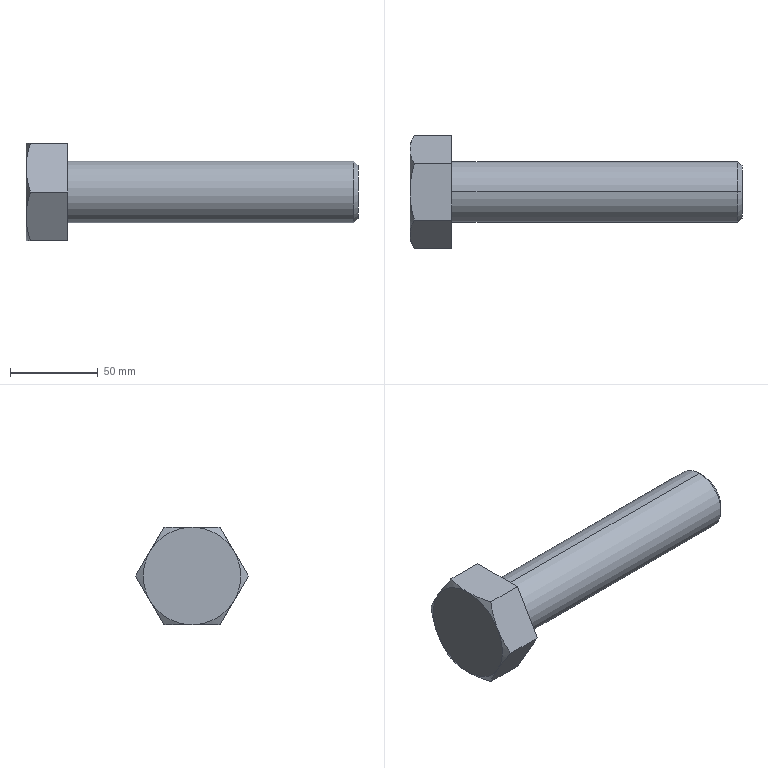Part | SolidWorks | features RevCut 2, Extrusion 1, Fillet 1, LPattern 1, Revolution 1 | 1 solid | 19 faces | box 188.976 x 64.173 x 55.575 mm | volume 221511 mm3 | plane 9 | cone 8 | cylinder 2 | commonest cylinder face diameters 34.925 x2
STEP:
#1=CARTESIAN_POINT('',(7.44,0.,0.5883));
#2=VERTEX_POINT('',#1);
#3=CARTESIAN_POINT('',(7.44,0.,-0.5883));
#4=VERTEX_POINT('',#3);
#5=CARTESIAN_POINT('',(7.44,0.,0.));
#6=DIRECTION('',(-1.,0.,0.));
#7=DIRECTION('',(0.,0.,1.));
#8=AXIS2_PLACEMENT_3D('',#5,#6,#7);
#9=CIRCLE('',#8,0.5883);
#10=EDGE_CURVE('',#2,#4,#9,.T.);
#11=ORIENTED_EDGE('',*,*,#10,.T.);
#12=CARTESIAN_POINT('',(7.341,0.,-0.6875));
#13=VERTEX_POINT('',#12);
#14=CARTESIAN_POINT('',(7.44,0.,-0.5883));
#15=DIRECTION('',(-0.7071,0.,-0.7071));
#16=VECTOR('',#15,39.37);
#17=LINE('',#14,#16);
#18=EDGE_CURVE('',#4,#13,#17,.T.);
#19=ORIENTED_EDGE('',*,*,#18,.T.);
#20=CARTESIAN_POINT('',(7.341,0.,0.6875));
#21=VERTEX_POINT('',#20);
#22=CARTESIAN_POINT('',(7.341,0.,0.));
#23=DIRECTION('',(-1.,0.,0.));
#24=DIRECTION('',(0.,0.,1.));
#25=AXIS2_PLACEMENT_3D('',#22,#23,#24);
#26=CIRCLE('',#25,0.6875);
#27=EDGE_CURVE('',#21,#13,#26,.T.);
#28=ORIENTED_EDGE('',*,*,#27,.F.);
#29=CARTESIAN_POINT('',(7.44,0.,0.5883));
#30=DIRECTION('',(-0.7071,0.,0.7071));
#31=VECTOR('',#30,39.37);
#32=LINE('',#29,#31);
#33=EDGE_CURVE('',#2,#21,#32,.T.);
#34=ORIENTED_EDGE('',*,*,#33,.F.);
#35=EDGE_LOOP('',(#11,#19,#28,#34));
#36=FACE_OUTER_BOUND('',#35,.T.);
#37=CARTESIAN_POINT('',(7.44,0.,0.));
#38=DIRECTION('',(-1.,0.,0.));
#39=DIRECTION('',(0.,0.,1.));
#40=AXIS2_PLACEMENT_3D('',#37,#38,#39);
#41=CONICAL_SURFACE('',#40,0.5883,0.7854);
#42=ADVANCED_FACE('',(#36),#41,.T.);
#43=ORIENTED_EDGE('',*,*,#27,.T.);
#44=CARTESIAN_POINT('',(0.94,0.,-0.6875));
#45=VERTEX_POINT('',#44);
#46=CARTESIAN_POINT('',(0.,0.,-0.6875));
#47=DIRECTION('',(-1.,0.,0.));
#48=VECTOR('',#47,39.37);
#49=LINE('',#46,#48);
#50=EDGE_CURVE('',#13,#45,#49,.T.);
#51=ORIENTED_EDGE('',*,*,#50,.T.);
#52=CARTESIAN_POINT('',(0.94,0.,0.6875));
#53=VERTEX_POINT('',#52);
#54=CARTESIAN_POINT('',(0.94,0.,0.));
#55=DIRECTION('',(-1.,0.,0.));
#56=DIRECTION('',(0.,0.,-1.));
#57=AXIS2_PLACEMENT_3D('',#54,#55,#56);
#58=CIRCLE('',#57,0.6875);
#59=EDGE_CURVE('',#53,#45,#58,.T.);
#60=ORIENTED_EDGE('',*,*,#59,.F.);
#61=CARTESIAN_POINT('',(0.,0.,0.6875));
#62=DIRECTION('',(-1.,0.,0.));
#63=VECTOR('',#62,39.37);
#64=LINE('',#61,#63);
#65=EDGE_CURVE('',#21,#53,#64,.T.);
#66=ORIENTED_EDGE('',*,*,#65,.F.);
#67=EDGE_LOOP('',(#43,#51,#60,#66));
#68=FACE_OUTER_BOUND('',#67,.T.);
#69=CARTESIAN_POINT('',(0.,0.,0.));
#70=DIRECTION('',(-1.,0.,0.));
#71=DIRECTION('',(0.,0.,1.));
#72=AXIS2_PLACEMENT_3D('',#69,#70,#71);
#73=CYLINDRICAL_SURFACE('',#72,0.6875);
#74=ADVANCED_FACE('',(#68),#73,.T.);
#75=CARTESIAN_POINT('',(0.09771,1.263,0.));
#76=VERTEX_POINT('',#75);
#77=CARTESIAN_POINT('',(0.,0.9474,-0.547));
#78=VERTEX_POINT('',#77);
#79=CARTESIAN_POINT('',(0.09771,1.263,0.));
#80=CARTESIAN_POINT('',(0.06788,1.212,-0.08948));
#81=CARTESIAN_POINT('',(0.04331,1.16,-0.1796));
#82=CARTESIAN_POINT('',(0.009312,1.054,-0.3618));
#83=CARTESIAN_POINT('',(0.,1.001,-0.4538));
#84=CARTESIAN_POINT('',(0.,0.9474,-0.547));
#85=B_SPLINE_CURVE_WITH_KNOTS('',3,(#79,#80,#81,#82,#83,#84),.UNSPECIFIED.,.F.,.F.,(4,2,4),(0.000000238,0.008117,0.01623),.UNSPECIFIED.);
#86=EDGE_CURVE('',#76,#78,#85,.T.);
#87=ORIENTED_EDGE('',*,*,#86,.F.);
#88=CARTESIAN_POINT('',(0.94,1.263,0.));
#89=VERTEX_POINT('',#88);
#90=CARTESIAN_POINT('',(0.94,1.263,0.));
#91=DIRECTION('',(-1.,0.,0.));
#92=VECTOR('',#91,39.37);
#93=LINE('',#90,#92);
#94=EDGE_CURVE('',#89,#76,#93,.T.);
#95=ORIENTED_EDGE('',*,*,#94,.F.);
#96=CARTESIAN_POINT('',(0.94,0.6316,-1.094));
#97=VERTEX_POINT('',#96);
#98=CARTESIAN_POINT('',(0.94,0.6316,-1.094));
#99=DIRECTION('',(0.,0.5,0.866));
#100=VECTOR('',#99,39.37);
#101=LINE('',#98,#100);
#102=EDGE_CURVE('',#97,#89,#101,.T.);
#103=ORIENTED_EDGE('',*,*,#102,.F.);
#104=CARTESIAN_POINT('',(0.09771,0.6316,-1.094));
#105=VERTEX_POINT('',#104);
#106=CARTESIAN_POINT('',(0.94,0.6316,-1.094));
#107=DIRECTION('',(-1.,0.,0.));
#108=VECTOR('',#107,39.37);
#109=LINE('',#106,#108);
#110=EDGE_CURVE('',#97,#105,#109,.T.);
#111=ORIENTED_EDGE('',*,*,#110,.T.);
#112=CARTESIAN_POINT('',(0.,0.9474,-0.547));
#113=CARTESIAN_POINT('',(0.,0.934,-0.5702));
#114=CARTESIAN_POINT('',(0.0005731,0.9206,-0.5935));
#115=CARTESIAN_POINT('',(0.002846,0.8938,-0.64));
#116=CARTESIAN_POINT('',(0.004544,0.8804,-0.6631));
#117=CARTESIAN_POINT('',(0.01125,0.8405,-0.7323));
#118=CARTESIAN_POINT('',(0.01787,0.814,-0.7781));
#119=CARTESIAN_POINT('',(0.0434,0.7351,-0.9147));
#120=CARTESIAN_POINT('',(0.06796,0.6832,-1.005));
#121=CARTESIAN_POINT('',(0.09771,0.6316,-1.094));
#122=B_SPLINE_CURVE_WITH_KNOTS('',3,(#112,#113,#114,#115,#116,#117,#118,#119,#120,#121),.UNSPECIFIED.,.F.,.F.,(4,2,2,2,4),(0.01623,0.01825,0.02028,0.02432,0.03241),.UNSPECIFIED.);
#123=EDGE_CURVE('',#78,#105,#122,.T.);
#124=ORIENTED_EDGE('',*,*,#123,.F.);
#125=EDGE_LOOP('',(#87,#95,#103,#111,#124));
#126=FACE_OUTER_BOUND('',#125,.T.);
#127=CARTESIAN_POINT('',(0.94,0.6316,-1.094));
#128=DIRECTION('',(0.,-0.866,0.5));
#129=DIRECTION('',(0.,-0.5,-0.866));
#130=AXIS2_PLACEMENT_3D('',#127,#128,#129);
#131=PLANE('',#130);
#132=ADVANCED_FACE('',(#126),#131,.F.);
#133=CARTESIAN_POINT('',(0.09771,0.6316,1.094));
#134=VERTEX_POINT('',#133);
#135=CARTESIAN_POINT('',(0.,0.9474,0.547));
#136=VERTEX_POINT('',#135);
#137=CARTESIAN_POINT('',(0.09771,0.6316,1.094));
#138=CARTESIAN_POINT('',(0.06788,0.6833,1.005));
#139=CARTESIAN_POINT('',(0.04331,0.7353,0.9144));
#140=CARTESIAN_POINT('',(0.009312,0.8405,0.7322));
#141=CARTESIAN_POINT('',(0.,0.8936,0.6402));
#142=CARTESIAN_POINT('',(0.,0.9474,0.547));
#143=B_SPLINE_CURVE_WITH_KNOTS('',3,(#137,#138,#139,#140,#141,#142),.UNSPECIFIED.,.F.,.F.,(4,2,4),(0.000000238,0.008117,0.01623),.UNSPECIFIED.);
#144=EDGE_CURVE('',#134,#136,#143,.T.);
#145=ORIENTED_EDGE('',*,*,#144,.F.);
#146=CARTESIAN_POINT('',(0.94,0.6316,1.094));
#147=VERTEX_POINT('',#146);
#148=CARTESIAN_POINT('',(0.94,0.6316,1.094));
#149=DIRECTION('',(-1.,0.,0.));
#150=VECTOR('',#149,39.37);
#151=LINE('',#148,#150);
#152=EDGE_CURVE('',#147,#134,#151,.T.);
#153=ORIENTED_EDGE('',*,*,#152,.F.);
#154=CARTESIAN_POINT('',(0.94,1.263,0.));
#155=DIRECTION('',(0.,-0.5,0.866));
#156=VECTOR('',#155,39.37);
#157=LINE('',#154,#156);
#158=EDGE_CURVE('',#89,#147,#157,.T.);
#159=ORIENTED_EDGE('',*,*,#158,.F.);
#160=ORIENTED_EDGE('',*,*,#94,.T.);
#161=CARTESIAN_POINT('',(0.,0.9474,0.547));
#162=CARTESIAN_POINT('',(0.,0.9608,0.5238));
#163=CARTESIAN_POINT('',(0.0005731,0.9743,0.5005));
#164=CARTESIAN_POINT('',(0.002846,1.001,0.454));
#165=CARTESIAN_POINT('',(0.004544,1.014,0.4309));
#166=CARTESIAN_POINT('',(0.01125,1.054,0.3617));
#167=CARTESIAN_POINT('',(0.01787,1.081,0.3159));
#168=CARTESIAN_POINT('',(0.0434,1.16,0.1793));
#169=CARTESIAN_POINT('',(0.06796,1.212,0.08926));
#170=CARTESIAN_POINT('',(0.09771,1.263,0.));
#171=B_SPLINE_CURVE_WITH_KNOTS('',3,(#161,#162,#163,#164,#165,#166,#167,#168,#169,#170),.UNSPECIFIED.,.F.,.F.,(4,2,2,2,4),(0.01623,0.01825,0.02028,0.02432,0.03241),.UNSPECIFIED.);
#172=EDGE_CURVE('',#136,#76,#171,.T.);
#173=ORIENTED_EDGE('',*,*,#172,.F.);
#174=EDGE_LOOP('',(#145,#153,#159,#160,#173));
#175=FACE_OUTER_BOUND('',#174,.T.);
#176=CARTESIAN_POINT('',(0.94,1.263,0.));
#177=DIRECTION('',(0.,-0.866,-0.5));
#178=DIRECTION('',(0.,0.5,-0.866));
#179=AXIS2_PLACEMENT_3D('',#176,#177,#178);
#180=PLANE('',#179);
#181=ADVANCED_FACE('',(#175),#180,.F.);
#182=CARTESIAN_POINT('',(0.09771,-0.6316,1.094));
#183=VERTEX_POINT('',#182);
#184=CARTESIAN_POINT('',(0.,0.,1.094));
#185=VERTEX_POINT('',#184);
#186=CARTESIAN_POINT('',(0.09771,-0.6316,1.094));
#187=CARTESIAN_POINT('',(0.08288,-0.5802,1.094));
#188=CARTESIAN_POINT('',(0.06924,-0.5283,1.094));
#189=CARTESIAN_POINT('',(0.0451,-0.4235,1.094));
#190=CARTESIAN_POINT('',(0.03468,-0.3709,1.094));
#191=CARTESIAN_POINT('',(0.009184,-0.2128,1.094));
#192=CARTESIAN_POINT('',(0.,-0.1068,1.094));
#193=CARTESIAN_POINT('',(0.,0.,1.094));
#194=B_SPLINE_CURVE_WITH_KNOTS('',3,(#186,#187,#188,#189,#190,#191,#192,#193),.UNSPECIFIED.,.F.,.F.,(4,2,2,4),(0.02919,0.03325,0.03731,0.04543),.UNSPECIFIED.);
#195=EDGE_CURVE('',#183,#185,#194,.T.);
#196=ORIENTED_EDGE('',*,*,#195,.F.);
#197=CARTESIAN_POINT('',(0.94,-0.6316,1.094));
#198=VERTEX_POINT('',#197);
#199=CARTESIAN_POINT('',(0.94,-0.6316,1.094));
#200=DIRECTION('',(-1.,0.,0.));
#201=VECTOR('',#200,39.37);
#202=LINE('',#199,#201);
#203=EDGE_CURVE('',#198,#183,#202,.T.);
#204=ORIENTED_EDGE('',*,*,#203,.F.);
#205=CARTESIAN_POINT('',(0.94,0.6316,1.094));
#206=DIRECTION('',(0.,-1.,0.));
#207=VECTOR('',#206,39.37);
#208=LINE('',#205,#207);
#209=EDGE_CURVE('',#147,#198,#208,.T.);
#210=ORIENTED_EDGE('',*,*,#209,.F.);
#211=ORIENTED_EDGE('',*,*,#152,.T.);
#212=CARTESIAN_POINT('',(0.,0.,1.094));
#213=CARTESIAN_POINT('',(0.,0.05344,1.094));
#214=CARTESIAN_POINT('',(0.002274,0.1071,1.094));
#215=CARTESIAN_POINT('',(0.01131,0.2147,1.094));
#216=CARTESIAN_POINT('',(0.018,0.2679,1.094));
#217=CARTESIAN_POINT('',(0.04368,0.426,1.094));
#218=CARTESIAN_POINT('',(0.06823,0.5295,1.094));
#219=CARTESIAN_POINT('',(0.09771,0.6316,1.094));
#220=B_SPLINE_CURVE_WITH_KNOTS('',3,(#212,#213,#214,#215,#216,#217,#218,#219),.UNSPECIFIED.,.F.,.F.,(4,2,2,4),(0.04543,0.04949,0.05355,0.06167),.UNSPECIFIED.);
#221=EDGE_CURVE('',#185,#134,#220,.T.);
#222=ORIENTED_EDGE('',*,*,#221,.F.);
#223=EDGE_LOOP('',(#196,#204,#210,#211,#222));
#224=FACE_OUTER_BOUND('',#223,.T.);
#225=CARTESIAN_POINT('',(0.94,0.6316,1.094));
#226=DIRECTION('',(0.,0.,-1.));
#227=DIRECTION('',(0.,1.,0.));
#228=AXIS2_PLACEMENT_3D('',#225,#226,#227);
#229=PLANE('',#228);
#230=ADVANCED_FACE('',(#224),#229,.F.);
#231=CARTESIAN_POINT('',(0.09771,-1.263,0.));
#232=VERTEX_POINT('',#231);
#233=CARTESIAN_POINT('',(0.,-0.9474,0.547));
#234=VERTEX_POINT('',#233);
#235=CARTESIAN_POINT('',(0.09771,-1.263,0.));
#236=CARTESIAN_POINT('',(0.06788,-1.212,0.08948));
#237=CARTESIAN_POINT('',(0.04331,-1.16,0.1796));
#238=CARTESIAN_POINT('',(0.009312,-1.054,0.3618));
#239=CARTESIAN_POINT('',(0.,-1.001,0.4538));
#240=CARTESIAN_POINT('',(0.,-0.9474,0.547));
#241=B_SPLINE_CURVE_WITH_KNOTS('',3,(#235,#236,#237,#238,#239,#240),.UNSPECIFIED.,.F.,.F.,(4,2,4),(0.000000238,0.008117,0.01623),.UNSPECIFIED.);
#242=EDGE_CURVE('',#232,#234,#241,.T.);
#243=ORIENTED_EDGE('',*,*,#242,.F.);
#244=CARTESIAN_POINT('',(0.94,-1.263,0.));
#245=VERTEX_POINT('',#244);
#246=CARTESIAN_POINT('',(0.94,-1.263,0.));
#247=DIRECTION('',(-1.,0.,0.));
#248=VECTOR('',#247,39.37);
#249=LINE('',#246,#248);
#250=EDGE_CURVE('',#245,#232,#249,.T.);
#251=ORIENTED_EDGE('',*,*,#250,.F.);
#252=CARTESIAN_POINT('',(0.94,-1.263,0.));
#253=DIRECTION('',(0.,-0.5,-0.866));
#254=VECTOR('',#253,39.37);
#255=LINE('',#252,#254);
#256=EDGE_CURVE('',#198,#245,#255,.T.);
#257=ORIENTED_EDGE('',*,*,#256,.F.);
#258=ORIENTED_EDGE('',*,*,#203,.T.);
#259=CARTESIAN_POINT('',(0.,-0.9474,0.547));
#260=CARTESIAN_POINT('',(0.,-0.934,0.5702));
#261=CARTESIAN_POINT('',(0.0005731,-0.9206,0.5935));
#262=CARTESIAN_POINT('',(0.002846,-0.8938,0.64));
#263=CARTESIAN_POINT('',(0.004544,-0.8804,0.6631));
#264=CARTESIAN_POINT('',(0.01125,-0.8405,0.7323));
#265=CARTESIAN_POINT('',(0.01787,-0.814,0.7781));
#266=CARTESIAN_POINT('',(0.0434,-0.7351,0.9147));
#267=CARTESIAN_POINT('',(0.06796,-0.6832,1.005));
#268=CARTESIAN_POINT('',(0.09771,-0.6316,1.094));
#269=B_SPLINE_CURVE_WITH_KNOTS('',3,(#259,#260,#261,#262,#263,#264,#265,#266,#267,#268),.UNSPECIFIED.,.F.,.F.,(4,2,2,2,4),(0.01623,0.01825,0.02028,0.02432,0.03241),.UNSPECIFIED.);
#270=EDGE_CURVE('',#234,#183,#269,.T.);
#271=ORIENTED_EDGE('',*,*,#270,.F.);
#272=EDGE_LOOP('',(#243,#251,#257,#258,#271));
#273=FACE_OUTER_BOUND('',#272,.T.);
#274=CARTESIAN_POINT('',(0.94,-1.263,0.));
#275=DIRECTION('',(0.,0.866,-0.5));
#276=DIRECTION('',(0.,0.5,0.866));
#277=AXIS2_PLACEMENT_3D('',#274,#275,#276);
#278=PLANE('',#277);
#279=ADVANCED_FACE('',(#273),#278,.F.);
#280=CARTESIAN_POINT('',(0.09771,-0.6316,-1.094));
#281=VERTEX_POINT('',#280);
#282=CARTESIAN_POINT('',(0.,-0.9474,-0.547));
#283=VERTEX_POINT('',#282);
#284=CARTESIAN_POINT('',(0.09771,-0.6316,-1.094));
#285=CARTESIAN_POINT('',(0.06788,-0.6833,-1.005));
#286=CARTESIAN_POINT('',(0.04331,-0.7353,-0.9144));
#287=CARTESIAN_POINT('',(0.009312,-0.8405,-0.7322));
#288=CARTESIAN_POINT('',(0.,-0.8936,-0.6402));
#289=CARTESIAN_POINT('',(0.,-0.9474,-0.547));
#290=B_SPLINE_CURVE_WITH_KNOTS('',3,(#284,#285,#286,#287,#288,#289),.UNSPECIFIED.,.F.,.F.,(4,2,4),(0.000000238,0.008117,0.01623),.UNSPECIFIED.);
#291=EDGE_CURVE('',#281,#283,#290,.T.);
#292=ORIENTED_EDGE('',*,*,#291,.F.);
#293=CARTESIAN_POINT('',(0.94,-0.6316,-1.094));
#294=VERTEX_POINT('',#293);
#295=CARTESIAN_POINT('',(0.94,-0.6316,-1.094));
#296=DIRECTION('',(-1.,0.,0.));
#297=VECTOR('',#296,39.37);
#298=LINE('',#295,#297);
#299=EDGE_CURVE('',#294,#281,#298,.T.);
#300=ORIENTED_EDGE('',*,*,#299,.F.);
#301=CARTESIAN_POINT('',(0.94,-0.6316,-1.094));
#302=DIRECTION('',(0.,0.5,-0.866));
#303=VECTOR('',#302,39.37);
#304=LINE('',#301,#303);
#305=EDGE_CURVE('',#245,#294,#304,.T.);
#306=ORIENTED_EDGE('',*,*,#305,.F.);
#307=ORIENTED_EDGE('',*,*,#250,.T.);
#308=CARTESIAN_POINT('',(0.,-0.9474,-0.547));
#309=CARTESIAN_POINT('',(0.,-0.9608,-0.5238));
#310=CARTESIAN_POINT('',(0.0005731,-0.9743,-0.5005));
#311=CARTESIAN_POINT('',(0.002846,-1.001,-0.454));
#312=CARTESIAN_POINT('',(0.004544,-1.014,-0.4309));
#313=CARTESIAN_POINT('',(0.01125,-1.054,-0.3617));
#314=CARTESIAN_POINT('',(0.01787,-1.081,-0.3159));
#315=CARTESIAN_POINT('',(0.0434,-1.16,-0.1793));
#316=CARTESIAN_POINT('',(0.06796,-1.212,-0.08926));
#317=CARTESIAN_POINT('',(0.09771,-1.263,0.));
#318=B_SPLINE_CURVE_WITH_KNOTS('',3,(#308,#309,#310,#311,#312,#313,#314,#315,#316,#317),.UNSPECIFIED.,.F.,.F.,(4,2,2,2,4),(0.01623,0.01825,0.02028,0.02432,0.03241),.UNSPECIFIED.);
#319=EDGE_CURVE('',#283,#232,#318,.T.);
#320=ORIENTED_EDGE('',*,*,#319,.F.);
#321=EDGE_LOOP('',(#292,#300,#306,#307,#320));
#322=FACE_OUTER_BOUND('',#321,.T.);
#323=CARTESIAN_POINT('',(0.94,-0.6316,-1.094));
#324=DIRECTION('',(0.,0.866,0.5));
#325=DIRECTION('',(0.,-0.5,0.866));
#326=AXIS2_PLACEMENT_3D('',#323,#324,#325);
#327=PLANE('',#326);
#328=ADVANCED_FACE('',(#322),#327,.F.);
#329=CARTESIAN_POINT('',(0.,0.,-1.094));
#330=VERTEX_POINT('',#329);
#331=CARTESIAN_POINT('',(0.09771,0.6316,-1.094));
#332=CARTESIAN_POINT('',(0.06823,0.5295,-1.094));
#333=CARTESIAN_POINT('',(0.04368,0.426,-1.094));
#334=CARTESIAN_POINT('',(0.018,0.2679,-1.094));
#335=CARTESIAN_POINT('',(0.01131,0.2147,-1.094));
#336=CARTESIAN_POINT('',(0.002274,0.1071,-1.094));
#337=CARTESIAN_POINT('',(0.,0.05344,-1.094));
#338=CARTESIAN_POINT('',(0.,0.,-1.094));
#339=B_SPLINE_CURVE_WITH_KNOTS('',3,(#331,#332,#333,#334,#335,#336,#337,#338),.UNSPECIFIED.,.F.,.F.,(4,2,2,4),(0.07205,0.08018,0.08424,0.08831),.UNSPECIFIED.);
#340=EDGE_CURVE('',#105,#330,#339,.T.);
#341=ORIENTED_EDGE('',*,*,#340,.F.);
#342=ORIENTED_EDGE('',*,*,#110,.F.);
#343=CARTESIAN_POINT('',(0.94,0.6316,-1.094));
#344=DIRECTION('',(0.,1.,0.));
#345=VECTOR('',#344,39.37);
#346=LINE('',#343,#345);
#347=EDGE_CURVE('',#294,#97,#346,.T.);
#348=ORIENTED_EDGE('',*,*,#347,.F.);
#349=ORIENTED_EDGE('',*,*,#299,.T.);
#350=CARTESIAN_POINT('',(0.,0.,-1.094));
#351=CARTESIAN_POINT('',(0.,-0.1068,-1.094));
#352=CARTESIAN_POINT('',(0.009184,-0.2128,-1.094));
#353=CARTESIAN_POINT('',(0.03468,-0.3709,-1.094));
#354=CARTESIAN_POINT('',(0.0451,-0.4235,-1.094));
#355=CARTESIAN_POINT('',(0.06924,-0.5283,-1.094));
#356=CARTESIAN_POINT('',(0.08288,-0.5802,-1.094));
#357=CARTESIAN_POINT('',(0.09771,-0.6316,-1.094));
#358=B_SPLINE_CURVE_WITH_KNOTS('',3,(#350,#351,#352,#353,#354,#355,#356,#357),.UNSPECIFIED.,.F.,.F.,(4,2,2,4),(0.08831,0.09643,0.1005,0.1046),.UNSPECIFIED.);
#359=EDGE_CURVE('',#330,#281,#358,.T.);
#360=ORIENTED_EDGE('',*,*,#359,.F.);
#361=EDGE_LOOP('',(#341,#342,#348,#349,#360));
#362=FACE_OUTER_BOUND('',#361,.T.);
#363=CARTESIAN_POINT('',(0.94,0.6316,-1.094));
#364=DIRECTION('',(0.,0.,1.));
#365=DIRECTION('',(0.,-1.,0.));
#366=AXIS2_PLACEMENT_3D('',#363,#364,#365);
#367=PLANE('',#366);
#368=ADVANCED_FACE('',(#362),#367,.F.);
#369=ORIENTED_EDGE('',*,*,#59,.T.);
#370=CARTESIAN_POINT('',(0.94,0.,0.));
#371=DIRECTION('',(-1.,0.,0.));
#372=DIRECTION('',(0.,0.,-1.));
#373=AXIS2_PLACEMENT_3D('',#370,#371,#372);
#374=CIRCLE('',#373,0.6875);
#375=EDGE_CURVE('',#45,#53,#374,.T.);
#376=ORIENTED_EDGE('',*,*,#375,.T.);
#377=EDGE_LOOP('',(#369,#376));
#378=FACE_BOUND('',#377,.T.);
#379=ORIENTED_EDGE('',*,*,#102,.T.);
#380=ORIENTED_EDGE('',*,*,#158,.T.);
#381=ORIENTED_EDGE('',*,*,#209,.T.);
#382=ORIENTED_EDGE('',*,*,#256,.T.);
#383=ORIENTED_EDGE('',*,*,#305,.T.);
#384=ORIENTED_EDGE('',*,*,#347,.T.);
#385=EDGE_LOOP('',(#379,#380,#381,#382,#383,#384));
#386=FACE_OUTER_BOUND('',#385,.T.);
#387=CARTESIAN_POINT('',(0.94,1.263,0.));
#388=DIRECTION('',(1.,0.,0.));
#389=DIRECTION('',(0.,0.,-1.));
#390=AXIS2_PLACEMENT_3D('',#387,#388,#389);
#391=PLANE('',#390);
#392=ADVANCED_FACE('',(#378,#386),#391,.T.);
#393=ORIENTED_EDGE('',*,*,#50,.F.);
#394=CARTESIAN_POINT('',(7.341,0.,0.));
#395=DIRECTION('',(-1.,0.,0.));
#396=DIRECTION('',(0.,0.,1.));
#397=AXIS2_PLACEMENT_3D('',#394,#395,#396);
#398=CIRCLE('',#397,0.6875);
#399=EDGE_CURVE('',#13,#21,#398,.T.);
#400=ORIENTED_EDGE('',*,*,#399,.T.);
#401=ORIENTED_EDGE('',*,*,#65,.T.);
#402=ORIENTED_EDGE('',*,*,#375,.F.);
#403=EDGE_LOOP('',(#393,#400,#401,#402));
#404=FACE_OUTER_BOUND('',#403,.T.);
#405=CARTESIAN_POINT('',(0.,0.,0.));
#406=DIRECTION('',(-1.,0.,0.));
#407=DIRECTION('',(0.,0.,1.));
#408=AXIS2_PLACEMENT_3D('',#405,#406,#407);
#409=CYLINDRICAL_SURFACE('',#408,0.6875);
#410=ADVANCED_FACE('',(#404),#409,.T.);
#411=ORIENTED_EDGE('',*,*,#18,.F.);
#412=CARTESIAN_POINT('',(7.44,0.,0.));
#413=DIRECTION('',(-1.,0.,0.));
#414=DIRECTION('',(0.,0.,1.));
#415=AXIS2_PLACEMENT_3D('',#412,#413,#414);
#416=CIRCLE('',#415,0.5883);
#417=EDGE_CURVE('',#4,#2,#416,.T.);
#418=ORIENTED_EDGE('',*,*,#417,.T.);
#419=ORIENTED_EDGE('',*,*,#33,.T.);
#420=ORIENTED_EDGE('',*,*,#399,.F.);
#421=EDGE_LOOP('',(#411,#418,#419,#420));
#422=FACE_OUTER_BOUND('',#421,.T.);
#423=CARTESIAN_POINT('',(7.44,0.,0.));
#424=DIRECTION('',(-1.,0.,0.));
#425=DIRECTION('',(0.,0.,1.));
#426=AXIS2_PLACEMENT_3D('',#423,#424,#425);
#427=CONICAL_SURFACE('',#426,0.5883,0.7854);
#428=ADVANCED_FACE('',(#422),#427,.T.);
#429=ORIENTED_EDGE('',*,*,#10,.F.);
#430=ORIENTED_EDGE('',*,*,#417,.F.);
#431=EDGE_LOOP('',(#429,#430));
#432=FACE_OUTER_BOUND('',#431,.T.);
#433=CARTESIAN_POINT('',(7.44,0.,0.));
#434=DIRECTION('',(-1.,0.,0.));
#435=DIRECTION('',(0.,0.,1.));
#436=AXIS2_PLACEMENT_3D('',#433,#434,#435);
#437=PLANE('',#436);
#438=ADVANCED_FACE('',(#432),#437,.F.);
#439=ORIENTED_EDGE('',*,*,#291,.T.);
#440=CARTESIAN_POINT('',(0.,0.,0.));
#441=DIRECTION('',(1.,0.,0.));
#442=DIRECTION('',(0.,0.,-1.));
#443=AXIS2_PLACEMENT_3D('',#440,#441,#442);
#444=CIRCLE('',#443,1.094);
#445=EDGE_CURVE('',#283,#330,#444,.T.);
#446=ORIENTED_EDGE('',*,*,#445,.T.);
#447=ORIENTED_EDGE('',*,*,#359,.T.);
#448=EDGE_LOOP('',(#439,#446,#447));
#449=FACE_OUTER_BOUND('',#448,.T.);
#450=CARTESIAN_POINT('',(0.,0.,0.));
#451=DIRECTION('',(1.,0.,0.));
#452=DIRECTION('',(0.,0.,-1.));
#453=AXIS2_PLACEMENT_3D('',#450,#451,#452);
#454=CONICAL_SURFACE('',#453,1.094,1.047);
#455=ADVANCED_FACE('',(#449),#454,.T.);
#456=ORIENTED_EDGE('',*,*,#242,.T.);
#457=CARTESIAN_POINT('',(0.,0.,0.));
#458=DIRECTION('',(1.,0.,0.));
#459=DIRECTION('',(0.,0.,-1.));
#460=AXIS2_PLACEMENT_3D('',#457,#458,#459);
#461=CIRCLE('',#460,1.094);
#462=EDGE_CURVE('',#234,#283,#461,.T.);
#463=ORIENTED_EDGE('',*,*,#462,.T.);
#464=ORIENTED_EDGE('',*,*,#319,.T.);
#465=EDGE_LOOP('',(#456,#463,#464));
#466=FACE_OUTER_BOUND('',#465,.T.);
#467=CARTESIAN_POINT('',(0.,0.,0.));
#468=DIRECTION('',(1.,0.,0.));
#469=DIRECTION('',(0.,0.,-1.));
#470=AXIS2_PLACEMENT_3D('',#467,#468,#469);
#471=CONICAL_SURFACE('',#470,1.094,1.047);
#472=ADVANCED_FACE('',(#466),#471,.T.);
#473=ORIENTED_EDGE('',*,*,#195,.T.);
#474=CARTESIAN_POINT('',(0.,0.,0.));
#475=DIRECTION('',(1.,0.,0.));
#476=DIRECTION('',(0.,0.,-1.));
#477=AXIS2_PLACEMENT_3D('',#474,#475,#476);
#478=CIRCLE('',#477,1.094);
#479=EDGE_CURVE('',#185,#234,#478,.T.);
#480=ORIENTED_EDGE('',*,*,#479,.T.);
#481=ORIENTED_EDGE('',*,*,#270,.T.);
#482=EDGE_LOOP('',(#473,#480,#481));
#483=FACE_OUTER_BOUND('',#482,.T.);
#484=CARTESIAN_POINT('',(0.,0.,0.));
#485=DIRECTION('',(1.,0.,0.));
#486=DIRECTION('',(0.,0.,-1.));
#487=AXIS2_PLACEMENT_3D('',#484,#485,#486);
#488=CONICAL_SURFACE('',#487,1.094,1.047);
#489=ADVANCED_FACE('',(#483),#488,.T.);
#490=ORIENTED_EDGE('',*,*,#221,.T.);
#491=ORIENTED_EDGE('',*,*,#144,.T.);
#492=CARTESIAN_POINT('',(0.,0.,0.));
#493=DIRECTION('',(-1.,0.,0.));
#494=DIRECTION('',(0.,0.,1.));
#495=AXIS2_PLACEMENT_3D('',#492,#493,#494);
#496=CIRCLE('',#495,1.094);
#497=EDGE_CURVE('',#185,#136,#496,.T.);
#498=ORIENTED_EDGE('',*,*,#497,.F.);
#499=EDGE_LOOP('',(#490,#491,#498));
#500=FACE_OUTER_BOUND('',#499,.T.);
#501=CARTESIAN_POINT('',(0.,0.,0.));
#502=DIRECTION('',(1.,0.,0.));
#503=DIRECTION('',(0.,0.,-1.));
#504=AXIS2_PLACEMENT_3D('',#501,#502,#503);
#505=CONICAL_SURFACE('',#504,1.094,1.047);
#506=ADVANCED_FACE('',(#500),#505,.T.);
#507=ORIENTED_EDGE('',*,*,#172,.T.);
#508=ORIENTED_EDGE('',*,*,#86,.T.);
#509=CARTESIAN_POINT('',(0.,0.,0.));
#510=DIRECTION('',(1.,0.,0.));
#511=DIRECTION('',(0.,0.,-1.));
#512=AXIS2_PLACEMENT_3D('',#509,#510,#511);
#513=CIRCLE('',#512,1.094);
#514=EDGE_CURVE('',#78,#136,#513,.T.);
#515=ORIENTED_EDGE('',*,*,#514,.T.);
#516=EDGE_LOOP('',(#507,#508,#515));
#517=FACE_OUTER_BOUND('',#516,.T.);
#518=CARTESIAN_POINT('',(0.,0.,0.));
#519=DIRECTION('',(1.,0.,0.));
#520=DIRECTION('',(0.,0.,-1.));
#521=AXIS2_PLACEMENT_3D('',#518,#519,#520);
#522=CONICAL_SURFACE('',#521,1.094,1.047);
#523=ADVANCED_FACE('',(#517),#522,.T.);
#524=ORIENTED_EDGE('',*,*,#123,.T.);
#525=ORIENTED_EDGE('',*,*,#340,.T.);
#526=CARTESIAN_POINT('',(0.,0.,0.));
#527=DIRECTION('',(1.,0.,0.));
#528=DIRECTION('',(0.,0.,-1.));
#529=AXIS2_PLACEMENT_3D('',#526,#527,#528);
#530=CIRCLE('',#529,1.094);
#531=EDGE_CURVE('',#330,#78,#530,.T.);
#532=ORIENTED_EDGE('',*,*,#531,.T.);
#533=EDGE_LOOP('',(#524,#525,#532));
#534=FACE_OUTER_BOUND('',#533,.T.);
#535=CARTESIAN_POINT('',(0.,0.,0.));
#536=DIRECTION('',(1.,0.,0.));
#537=DIRECTION('',(0.,0.,-1.));
#538=AXIS2_PLACEMENT_3D('',#535,#536,#537);
#539=CONICAL_SURFACE('',#538,1.094,1.047);
#540=ADVANCED_FACE('',(#534),#539,.T.);
#541=ORIENTED_EDGE('',*,*,#531,.F.);
#542=ORIENTED_EDGE('',*,*,#445,.F.);
#543=ORIENTED_EDGE('',*,*,#462,.F.);
#544=ORIENTED_EDGE('',*,*,#479,.F.);
#545=ORIENTED_EDGE('',*,*,#497,.T.);
#546=ORIENTED_EDGE('',*,*,#514,.F.);
#547=EDGE_LOOP('',(#541,#542,#543,#544,#545,#546));
#548=FACE_OUTER_BOUND('',#547,.T.);
#549=CARTESIAN_POINT('',(0.,1.263,0.));
#550=DIRECTION('',(1.,0.,0.));
#551=DIRECTION('',(0.,0.,-1.));
#552=AXIS2_PLACEMENT_3D('',#549,#550,#551);
#553=PLANE('',#552);
#554=ADVANCED_FACE('',(#548),#553,.F.);
#555=CLOSED_SHELL('',(#42,#74,#132,#181,#230,#279,#328,#368,#392,#410,#428,#438,#455,#472,#489,#506,#523,#540,#554));
#556=MANIFOLD_SOLID_BREP('',#555);
#557=CARTESIAN_POINT('',(0.,0.,0.));
#558=DIRECTION('',(0.,0.,1.));
#559=DIRECTION('',(1.,0.,0.));
#560=AXIS2_PLACEMENT_3D('',#557,#558,#559);
#561=(LENGTH_UNIT()NAMED_UNIT(*)SI_UNIT($,.METRE.));
#562=LENGTH_MEASURE_WITH_UNIT(LENGTH_MEASURE(0.0254),#561);
#563=DIMENSIONAL_EXPONENTS(1.,0.,0.,0.,0.,0.,0.);
#564=(CONVERSION_BASED_UNIT('INCH',#562)LENGTH_UNIT()NAMED_UNIT(#563));
#565=UNCERTAINTY_MEASURE_WITH_UNIT(LENGTH_MEASURE(0.00001),#564,'','');
#566=(NAMED_UNIT(*)PLANE_ANGLE_UNIT()SI_UNIT($,.RADIAN.));
#567=(NAMED_UNIT(*)SI_UNIT($,.STERADIAN.)SOLID_ANGLE_UNIT());
#568=(GEOMETRIC_REPRESENTATION_CONTEXT(3)GLOBAL_UNCERTAINTY_ASSIGNED_CONTEXT((#565))GLOBAL_UNIT_ASSIGNED_CONTEXT((#564,#566,#567))REPRESENTATION_CONTEXT('',''));
#569=ADVANCED_BREP_SHAPE_REPRESENTATION('',(#556,#560),#568);